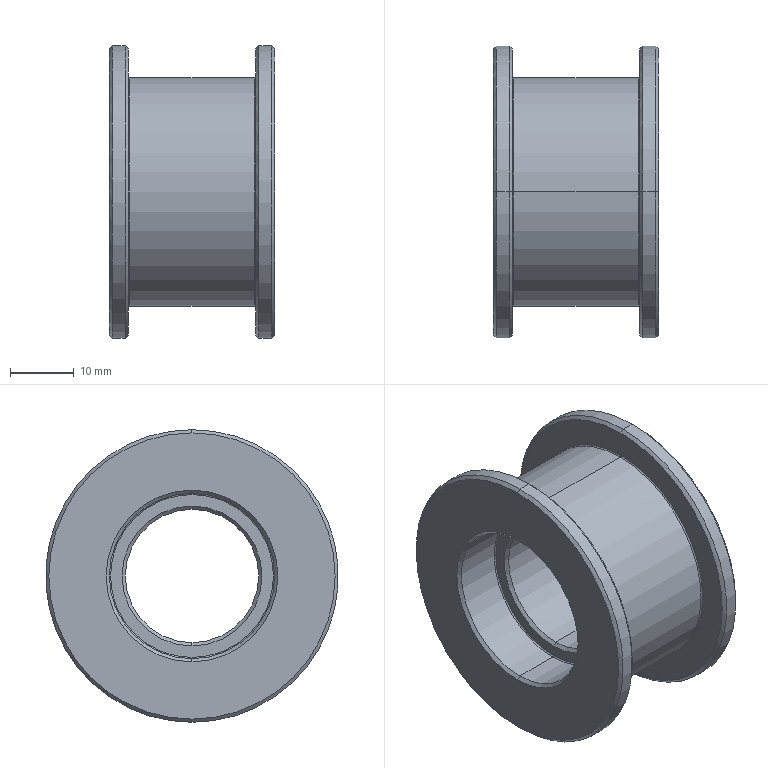Part | SolidWorks | features Chamfer 1, Fillet 1, Revolution 1 | 1 solid | 42 faces | box 26 x 46 x 46 mm | volume 18265 mm3 | cone 16 | cylinder 12 | torus 8 | plane 6 | commonest cylinder face diameters 26 x4 46 x4 21 x2 36 x2
STEP:
#1=CARTESIAN_POINT('',(-5.2,0.,13.));
#2=VERTEX_POINT('',#1);
#3=CARTESIAN_POINT('',(-5.2,0.,-13.));
#4=VERTEX_POINT('',#3);
#5=CARTESIAN_POINT('',(-5.2,0.,0.));
#6=DIRECTION('',(1.,0.,0.));
#7=DIRECTION('',(0.,0.,-1.));
#8=AXIS2_PLACEMENT_3D('',#5,#6,#7);
#9=CIRCLE('',#8,13.);
#10=EDGE_CURVE('',#2,#4,#9,.T.);
#11=ORIENTED_EDGE('',*,*,#10,.F.);
#12=CARTESIAN_POINT('',(-5.,0.,12.8));
#13=VERTEX_POINT('',#12);
#14=CARTESIAN_POINT('',(-5.2,0.,12.8));
#15=DIRECTION('',(0.,1.,0.));
#16=DIRECTION('',(0.,0.,1.));
#17=AXIS2_PLACEMENT_3D('',#14,#15,#16);
#18=CIRCLE('',#17,0.2);
#19=EDGE_CURVE('',#2,#13,#18,.T.);
#20=ORIENTED_EDGE('',*,*,#19,.T.);
#21=CARTESIAN_POINT('',(-5.,0.,-12.8));
#22=VERTEX_POINT('',#21);
#23=CARTESIAN_POINT('',(-5.,0.,0.));
#24=DIRECTION('',(-1.,0.,0.));
#25=DIRECTION('',(0.,0.,-1.));
#26=AXIS2_PLACEMENT_3D('',#23,#24,#25);
#27=CIRCLE('',#26,12.8);
#28=EDGE_CURVE('',#22,#13,#27,.T.);
#29=ORIENTED_EDGE('',*,*,#28,.F.);
#30=CARTESIAN_POINT('',(-5.2,0.,-12.8));
#31=DIRECTION('',(0.,-1.,0.));
#32=DIRECTION('',(0.,0.,-1.));
#33=AXIS2_PLACEMENT_3D('',#30,#31,#32);
#34=CIRCLE('',#33,0.2);
#35=EDGE_CURVE('',#4,#22,#34,.T.);
#36=ORIENTED_EDGE('',*,*,#35,.F.);
#37=EDGE_LOOP('',(#11,#20,#29,#36));
#38=FACE_OUTER_BOUND('',#37,.T.);
#39=CARTESIAN_POINT('',(-5.2,0.,0.));
#40=DIRECTION('',(1.,0.,0.));
#41=DIRECTION('',(0.,0.,-1.));
#42=AXIS2_PLACEMENT_3D('',#39,#40,#41);
#43=TOROIDAL_SURFACE('',#42,12.8,0.2);
#44=ADVANCED_FACE('',(#38),#43,.F.);
#45=CARTESIAN_POINT('',(10.,0.,18.2));
#46=VERTEX_POINT('',#45);
#47=CARTESIAN_POINT('',(10.,0.,-18.2));
#48=VERTEX_POINT('',#47);
#49=CARTESIAN_POINT('',(10.,0.,0.));
#50=DIRECTION('',(1.,0.,0.));
#51=DIRECTION('',(0.,0.,-1.));
#52=AXIS2_PLACEMENT_3D('',#49,#50,#51);
#53=CIRCLE('',#52,18.2);
#54=EDGE_CURVE('',#46,#48,#53,.T.);
#55=ORIENTED_EDGE('',*,*,#54,.F.);
#56=CARTESIAN_POINT('',(9.8,0.,18.));
#57=VERTEX_POINT('',#56);
#58=CARTESIAN_POINT('',(9.8,0.,18.2));
#59=DIRECTION('',(0.,1.,0.));
#60=DIRECTION('',(0.,0.,1.));
#61=AXIS2_PLACEMENT_3D('',#58,#59,#60);
#62=CIRCLE('',#61,0.2);
#63=EDGE_CURVE('',#46,#57,#62,.T.);
#64=ORIENTED_EDGE('',*,*,#63,.T.);
#65=CARTESIAN_POINT('',(9.8,0.,-18.));
#66=VERTEX_POINT('',#65);
#67=CARTESIAN_POINT('',(9.8,0.,0.));
#68=DIRECTION('',(-1.,0.,0.));
#69=DIRECTION('',(0.,0.,-1.));
#70=AXIS2_PLACEMENT_3D('',#67,#68,#69);
#71=CIRCLE('',#70,18.);
#72=EDGE_CURVE('',#66,#57,#71,.T.);
#73=ORIENTED_EDGE('',*,*,#72,.F.);
#74=CARTESIAN_POINT('',(9.8,0.,-18.2));
#75=DIRECTION('',(0.,-1.,0.));
#76=DIRECTION('',(0.,0.,-1.));
#77=AXIS2_PLACEMENT_3D('',#74,#75,#76);
#78=CIRCLE('',#77,0.2);
#79=EDGE_CURVE('',#48,#66,#78,.T.);
#80=ORIENTED_EDGE('',*,*,#79,.F.);
#81=EDGE_LOOP('',(#55,#64,#73,#80));
#82=FACE_OUTER_BOUND('',#81,.T.);
#83=CARTESIAN_POINT('',(9.8,0.,0.));
#84=DIRECTION('',(1.,0.,0.));
#85=DIRECTION('',(0.,0.,-1.));
#86=AXIS2_PLACEMENT_3D('',#83,#84,#85);
#87=TOROIDAL_SURFACE('',#86,18.2,0.2);
#88=ADVANCED_FACE('',(#82),#87,.F.);
#89=CARTESIAN_POINT('',(-10.,0.,-18.2));
#90=VERTEX_POINT('',#89);
#91=CARTESIAN_POINT('',(-10.,0.,18.2));
#92=VERTEX_POINT('',#91);
#93=CARTESIAN_POINT('',(-10.,0.,0.));
#94=DIRECTION('',(-1.,0.,0.));
#95=DIRECTION('',(0.,0.,1.));
#96=AXIS2_PLACEMENT_3D('',#93,#94,#95);
#97=CIRCLE('',#96,18.2);
#98=EDGE_CURVE('',#90,#92,#97,.T.);
#99=ORIENTED_EDGE('',*,*,#98,.F.);
#100=CARTESIAN_POINT('',(-9.8,0.,-18.));
#101=VERTEX_POINT('',#100);
#102=CARTESIAN_POINT('',(-9.8,0.,-18.2));
#103=DIRECTION('',(0.,1.,0.));
#104=DIRECTION('',(0.,0.,1.));
#105=AXIS2_PLACEMENT_3D('',#102,#103,#104);
#106=CIRCLE('',#105,0.2);
#107=EDGE_CURVE('',#90,#101,#106,.T.);
#108=ORIENTED_EDGE('',*,*,#107,.T.);
#109=CARTESIAN_POINT('',(-9.8,0.,18.));
#110=VERTEX_POINT('',#109);
#111=CARTESIAN_POINT('',(-9.8,0.,0.));
#112=DIRECTION('',(1.,0.,0.));
#113=DIRECTION('',(0.,0.,1.));
#114=AXIS2_PLACEMENT_3D('',#111,#112,#113);
#115=CIRCLE('',#114,18.);
#116=EDGE_CURVE('',#110,#101,#115,.T.);
#117=ORIENTED_EDGE('',*,*,#116,.F.);
#118=CARTESIAN_POINT('',(-9.8,0.,18.2));
#119=DIRECTION('',(0.,-1.,0.));
#120=DIRECTION('',(0.,0.,-1.));
#121=AXIS2_PLACEMENT_3D('',#118,#119,#120);
#122=CIRCLE('',#121,0.2);
#123=EDGE_CURVE('',#92,#110,#122,.T.);
#124=ORIENTED_EDGE('',*,*,#123,.F.);
#125=EDGE_LOOP('',(#99,#108,#117,#124));
#126=FACE_OUTER_BOUND('',#125,.T.);
#127=CARTESIAN_POINT('',(-9.8,0.,0.));
#128=DIRECTION('',(-1.,0.,0.));
#129=DIRECTION('',(0.,0.,1.));
#130=AXIS2_PLACEMENT_3D('',#127,#128,#129);
#131=TOROIDAL_SURFACE('',#130,18.2,0.2);
#132=ADVANCED_FACE('',(#126),#131,.F.);
#133=CARTESIAN_POINT('',(5.2,0.,-13.));
#134=VERTEX_POINT('',#133);
#135=CARTESIAN_POINT('',(5.2,0.,13.));
#136=VERTEX_POINT('',#135);
#137=CARTESIAN_POINT('',(5.2,0.,0.));
#138=DIRECTION('',(-1.,0.,0.));
#139=DIRECTION('',(0.,0.,1.));
#140=AXIS2_PLACEMENT_3D('',#137,#138,#139);
#141=CIRCLE('',#140,13.);
#142=EDGE_CURVE('',#134,#136,#141,.T.);
#143=ORIENTED_EDGE('',*,*,#142,.F.);
#144=CARTESIAN_POINT('',(5.,0.,-12.8));
#145=VERTEX_POINT('',#144);
#146=CARTESIAN_POINT('',(5.2,0.,-12.8));
#147=DIRECTION('',(0.,1.,0.));
#148=DIRECTION('',(0.,0.,1.));
#149=AXIS2_PLACEMENT_3D('',#146,#147,#148);
#150=CIRCLE('',#149,0.2);
#151=EDGE_CURVE('',#134,#145,#150,.T.);
#152=ORIENTED_EDGE('',*,*,#151,.T.);
#153=CARTESIAN_POINT('',(5.,0.,12.8));
#154=VERTEX_POINT('',#153);
#155=CARTESIAN_POINT('',(5.,0.,0.));
#156=DIRECTION('',(1.,0.,0.));
#157=DIRECTION('',(0.,0.,1.));
#158=AXIS2_PLACEMENT_3D('',#155,#156,#157);
#159=CIRCLE('',#158,12.8);
#160=EDGE_CURVE('',#154,#145,#159,.T.);
#161=ORIENTED_EDGE('',*,*,#160,.F.);
#162=CARTESIAN_POINT('',(5.2,0.,12.8));
#163=DIRECTION('',(0.,-1.,0.));
#164=DIRECTION('',(0.,0.,-1.));
#165=AXIS2_PLACEMENT_3D('',#162,#163,#164);
#166=CIRCLE('',#165,0.2);
#167=EDGE_CURVE('',#136,#154,#166,.T.);
#168=ORIENTED_EDGE('',*,*,#167,.F.);
#169=EDGE_LOOP('',(#143,#152,#161,#168));
#170=FACE_OUTER_BOUND('',#169,.T.);
#171=CARTESIAN_POINT('',(5.2,0.,0.));
#172=DIRECTION('',(-1.,0.,0.));
#173=DIRECTION('',(0.,0.,1.));
#174=AXIS2_PLACEMENT_3D('',#171,#172,#173);
#175=TOROIDAL_SURFACE('',#174,12.8,0.2);
#176=ADVANCED_FACE('',(#170),#175,.F.);
#177=CARTESIAN_POINT('',(-13.,0.,22.5));
#178=VERTEX_POINT('',#177);
#179=CARTESIAN_POINT('',(-13.,0.,-22.5));
#180=VERTEX_POINT('',#179);
#181=CARTESIAN_POINT('',(-13.,0.,0.));
#182=DIRECTION('',(-1.,0.,0.));
#183=DIRECTION('',(0.,0.,-1.));
#184=AXIS2_PLACEMENT_3D('',#181,#182,#183);
#185=CIRCLE('',#184,22.5);
#186=EDGE_CURVE('',#178,#180,#185,.T.);
#187=ORIENTED_EDGE('',*,*,#186,.F.);
#188=CARTESIAN_POINT('',(-12.5,0.,23.));
#189=VERTEX_POINT('',#188);
#190=CARTESIAN_POINT('',(-13.,0.,22.5));
#191=DIRECTION('',(0.7071,0.,0.7071));
#192=VECTOR('',#191,1000.);
#193=LINE('',#190,#192);
#194=EDGE_CURVE('',#178,#189,#193,.T.);
#195=ORIENTED_EDGE('',*,*,#194,.T.);
#196=CARTESIAN_POINT('',(-12.5,0.,-23.));
#197=VERTEX_POINT('',#196);
#198=CARTESIAN_POINT('',(-12.5,0.,0.));
#199=DIRECTION('',(1.,0.,0.));
#200=DIRECTION('',(0.,0.,-1.));
#201=AXIS2_PLACEMENT_3D('',#198,#199,#200);
#202=CIRCLE('',#201,23.);
#203=EDGE_CURVE('',#197,#189,#202,.T.);
#204=ORIENTED_EDGE('',*,*,#203,.F.);
#205=CARTESIAN_POINT('',(-13.,0.,-22.5));
#206=DIRECTION('',(0.7071,0.,-0.7071));
#207=VECTOR('',#206,1000.);
#208=LINE('',#205,#207);
#209=EDGE_CURVE('',#180,#197,#208,.T.);
#210=ORIENTED_EDGE('',*,*,#209,.F.);
#211=EDGE_LOOP('',(#187,#195,#204,#210));
#212=FACE_OUTER_BOUND('',#211,.T.);
#213=CARTESIAN_POINT('',(-13.,0.,0.));
#214=DIRECTION('',(1.,0.,0.));
#215=DIRECTION('',(0.,0.,-1.));
#216=AXIS2_PLACEMENT_3D('',#213,#214,#215);
#217=CONICAL_SURFACE('',#216,22.5,0.7854);
#218=ADVANCED_FACE('',(#212),#217,.T.);
#219=CARTESIAN_POINT('',(-12.5,0.,-13.));
#220=VERTEX_POINT('',#219);
#221=CARTESIAN_POINT('',(-12.5,0.,13.));
#222=VERTEX_POINT('',#221);
#223=CARTESIAN_POINT('',(-12.5,0.,0.));
#224=DIRECTION('',(-1.,0.,0.));
#225=DIRECTION('',(0.,0.,-1.));
#226=AXIS2_PLACEMENT_3D('',#223,#224,#225);
#227=CIRCLE('',#226,13.);
#228=EDGE_CURVE('',#220,#222,#227,.T.);
#229=ORIENTED_EDGE('',*,*,#228,.F.);
#230=CARTESIAN_POINT('',(-13.,0.,-13.5));
#231=VERTEX_POINT('',#230);
#232=CARTESIAN_POINT('',(-12.5,0.,-13.));
#233=DIRECTION('',(-0.7071,0.,-0.7071));
#234=VECTOR('',#233,1000.);
#235=LINE('',#232,#234);
#236=EDGE_CURVE('',#220,#231,#235,.T.);
#237=ORIENTED_EDGE('',*,*,#236,.T.);
#238=CARTESIAN_POINT('',(-13.,0.,13.5));
#239=VERTEX_POINT('',#238);
#240=CARTESIAN_POINT('',(-13.,0.,0.));
#241=DIRECTION('',(1.,0.,0.));
#242=DIRECTION('',(0.,0.,-1.));
#243=AXIS2_PLACEMENT_3D('',#240,#241,#242);
#244=CIRCLE('',#243,13.5);
#245=EDGE_CURVE('',#239,#231,#244,.T.);
#246=ORIENTED_EDGE('',*,*,#245,.F.);
#247=CARTESIAN_POINT('',(-12.5,0.,13.));
#248=DIRECTION('',(-0.7071,0.,0.7071));
#249=VECTOR('',#248,1000.);
#250=LINE('',#247,#249);
#251=EDGE_CURVE('',#222,#239,#250,.T.);
#252=ORIENTED_EDGE('',*,*,#251,.F.);
#253=EDGE_LOOP('',(#229,#237,#246,#252));
#254=FACE_OUTER_BOUND('',#253,.T.);
#255=CARTESIAN_POINT('',(-12.5,0.,0.));
#256=DIRECTION('',(-1.,0.,0.));
#257=DIRECTION('',(0.,0.,1.));
#258=AXIS2_PLACEMENT_3D('',#255,#256,#257);
#259=CONICAL_SURFACE('',#258,13.,0.7854);
#260=ADVANCED_FACE('',(#254),#259,.F.);
#261=CARTESIAN_POINT('',(-4.5,0.,-10.5));
#262=VERTEX_POINT('',#261);
#263=CARTESIAN_POINT('',(-4.5,0.,10.5));
#264=VERTEX_POINT('',#263);
#265=CARTESIAN_POINT('',(-4.5,0.,0.));
#266=DIRECTION('',(-1.,0.,0.));
#267=DIRECTION('',(0.,0.,-1.));
#268=AXIS2_PLACEMENT_3D('',#265,#266,#267);
#269=CIRCLE('',#268,10.5);
#270=EDGE_CURVE('',#262,#264,#269,.T.);
#271=ORIENTED_EDGE('',*,*,#270,.F.);
#272=CARTESIAN_POINT('',(-5.,0.,-11.));
#273=VERTEX_POINT('',#272);
#274=CARTESIAN_POINT('',(-4.5,0.,-10.5));
#275=DIRECTION('',(-0.7071,0.,-0.7071));
#276=VECTOR('',#275,1000.);
#277=LINE('',#274,#276);
#278=EDGE_CURVE('',#262,#273,#277,.T.);
#279=ORIENTED_EDGE('',*,*,#278,.T.);
#280=CARTESIAN_POINT('',(-5.,0.,11.));
#281=VERTEX_POINT('',#280);
#282=CARTESIAN_POINT('',(-5.,0.,0.));
#283=DIRECTION('',(1.,0.,0.));
#284=DIRECTION('',(0.,0.,-1.));
#285=AXIS2_PLACEMENT_3D('',#282,#283,#284);
#286=CIRCLE('',#285,11.);
#287=EDGE_CURVE('',#281,#273,#286,.T.);
#288=ORIENTED_EDGE('',*,*,#287,.F.);
#289=CARTESIAN_POINT('',(-4.5,0.,10.5));
#290=DIRECTION('',(-0.7071,0.,0.7071));
#291=VECTOR('',#290,1000.);
#292=LINE('',#289,#291);
#293=EDGE_CURVE('',#264,#281,#292,.T.);
#294=ORIENTED_EDGE('',*,*,#293,.F.);
#295=EDGE_LOOP('',(#271,#279,#288,#294));
#296=FACE_OUTER_BOUND('',#295,.T.);
#297=CARTESIAN_POINT('',(-4.5,0.,0.));
#298=DIRECTION('',(-1.,0.,0.));
#299=DIRECTION('',(0.,0.,1.));
#300=AXIS2_PLACEMENT_3D('',#297,#298,#299);
#301=CONICAL_SURFACE('',#300,10.5,0.7854);
#302=ADVANCED_FACE('',(#296),#301,.F.);
#303=CARTESIAN_POINT('',(-10.,0.,-22.5));
#304=VERTEX_POINT('',#303);
#305=CARTESIAN_POINT('',(-10.,0.,22.5));
#306=VERTEX_POINT('',#305);
#307=CARTESIAN_POINT('',(-10.,0.,0.));
#308=DIRECTION('',(1.,0.,0.));
#309=DIRECTION('',(0.,0.,1.));
#310=AXIS2_PLACEMENT_3D('',#307,#308,#309);
#311=CIRCLE('',#310,22.5);
#312=EDGE_CURVE('',#304,#306,#311,.T.);
#313=ORIENTED_EDGE('',*,*,#312,.F.);
#314=CARTESIAN_POINT('',(-10.5,0.,-23.));
#315=VERTEX_POINT('',#314);
#316=CARTESIAN_POINT('',(-10.5,0.,-23.));
#317=DIRECTION('',(-0.7071,0.,-0.7071));
#318=VECTOR('',#317,1000.);
#319=LINE('',#316,#318);
#320=EDGE_CURVE('',#304,#315,#319,.T.);
#321=ORIENTED_EDGE('',*,*,#320,.T.);
#322=CARTESIAN_POINT('',(-10.5,0.,23.));
#323=VERTEX_POINT('',#322);
#324=CARTESIAN_POINT('',(-10.5,0.,0.));
#325=DIRECTION('',(-1.,0.,0.));
#326=DIRECTION('',(0.,0.,1.));
#327=AXIS2_PLACEMENT_3D('',#324,#325,#326);
#328=CIRCLE('',#327,23.);
#329=EDGE_CURVE('',#323,#315,#328,.T.);
#330=ORIENTED_EDGE('',*,*,#329,.F.);
#331=CARTESIAN_POINT('',(-10.5,0.,23.));
#332=DIRECTION('',(-0.7071,0.,0.7071));
#333=VECTOR('',#332,1000.);
#334=LINE('',#331,#333);
#335=EDGE_CURVE('',#306,#323,#334,.T.);
#336=ORIENTED_EDGE('',*,*,#335,.F.);
#337=EDGE_LOOP('',(#313,#321,#330,#336));
#338=FACE_OUTER_BOUND('',#337,.T.);
#339=CARTESIAN_POINT('',(-10.5,0.,0.));
#340=DIRECTION('',(-1.,0.,0.));
#341=DIRECTION('',(0.,0.,1.));
#342=AXIS2_PLACEMENT_3D('',#339,#340,#341);
#343=CONICAL_SURFACE('',#342,23.,0.7854);
#344=ADVANCED_FACE('',(#338),#343,.T.);
#345=CARTESIAN_POINT('',(10.,0.,22.5));
#346=VERTEX_POINT('',#345);
#347=CARTESIAN_POINT('',(10.,0.,-22.5));
#348=VERTEX_POINT('',#347);
#349=CARTESIAN_POINT('',(10.,0.,0.));
#350=DIRECTION('',(-1.,0.,0.));
#351=DIRECTION('',(0.,0.,-1.));
#352=AXIS2_PLACEMENT_3D('',#349,#350,#351);
#353=CIRCLE('',#352,22.5);
#354=EDGE_CURVE('',#346,#348,#353,.T.);
#355=ORIENTED_EDGE('',*,*,#354,.F.);
#356=CARTESIAN_POINT('',(10.5,0.,23.));
#357=VERTEX_POINT('',#356);
#358=CARTESIAN_POINT('',(10.,0.,22.5));
#359=DIRECTION('',(0.7071,0.,0.7071));
#360=VECTOR('',#359,1000.);
#361=LINE('',#358,#360);
#362=EDGE_CURVE('',#346,#357,#361,.T.);
#363=ORIENTED_EDGE('',*,*,#362,.T.);
#364=CARTESIAN_POINT('',(10.5,0.,-23.));
#365=VERTEX_POINT('',#364);
#366=CARTESIAN_POINT('',(10.5,0.,0.));
#367=DIRECTION('',(1.,0.,0.));
#368=DIRECTION('',(0.,0.,-1.));
#369=AXIS2_PLACEMENT_3D('',#366,#367,#368);
#370=CIRCLE('',#369,23.);
#371=EDGE_CURVE('',#365,#357,#370,.T.);
#372=ORIENTED_EDGE('',*,*,#371,.F.);
#373=CARTESIAN_POINT('',(10.,0.,-22.5));
#374=DIRECTION('',(0.7071,0.,-0.7071));
#375=VECTOR('',#374,1000.);
#376=LINE('',#373,#375);
#377=EDGE_CURVE('',#348,#365,#376,.T.);
#378=ORIENTED_EDGE('',*,*,#377,.F.);
#379=EDGE_LOOP('',(#355,#363,#372,#378));
#380=FACE_OUTER_BOUND('',#379,.T.);
#381=CARTESIAN_POINT('',(10.,0.,0.));
#382=DIRECTION('',(1.,0.,0.));
#383=DIRECTION('',(0.,0.,-1.));
#384=AXIS2_PLACEMENT_3D('',#381,#382,#383);
#385=CONICAL_SURFACE('',#384,22.5,0.7854);
#386=ADVANCED_FACE('',(#380),#385,.T.);
#387=CARTESIAN_POINT('',(13.,0.,-22.5));
#388=VERTEX_POINT('',#387);
#389=CARTESIAN_POINT('',(13.,0.,22.5));
#390=VERTEX_POINT('',#389);
#391=CARTESIAN_POINT('',(13.,0.,0.));
#392=DIRECTION('',(1.,0.,0.));
#393=DIRECTION('',(0.,0.,1.));
#394=AXIS2_PLACEMENT_3D('',#391,#392,#393);
#395=CIRCLE('',#394,22.5);
#396=EDGE_CURVE('',#388,#390,#395,.T.);
#397=ORIENTED_EDGE('',*,*,#396,.F.);
#398=CARTESIAN_POINT('',(12.5,0.,-23.));
#399=VERTEX_POINT('',#398);
#400=CARTESIAN_POINT('',(12.5,0.,-23.));
#401=DIRECTION('',(-0.7071,0.,-0.7071));
#402=VECTOR('',#401,1000.);
#403=LINE('',#400,#402);
#404=EDGE_CURVE('',#388,#399,#403,.T.);
#405=ORIENTED_EDGE('',*,*,#404,.T.);
#406=CARTESIAN_POINT('',(12.5,0.,23.));
#407=VERTEX_POINT('',#406);
#408=CARTESIAN_POINT('',(12.5,0.,0.));
#409=DIRECTION('',(-1.,0.,0.));
#410=DIRECTION('',(0.,0.,1.));
#411=AXIS2_PLACEMENT_3D('',#408,#409,#410);
#412=CIRCLE('',#411,23.);
#413=EDGE_CURVE('',#407,#399,#412,.T.);
#414=ORIENTED_EDGE('',*,*,#413,.F.);
#415=CARTESIAN_POINT('',(12.5,0.,23.));
#416=DIRECTION('',(-0.7071,0.,0.7071));
#417=VECTOR('',#416,1000.);
#418=LINE('',#415,#417);
#419=EDGE_CURVE('',#390,#407,#418,.T.);
#420=ORIENTED_EDGE('',*,*,#419,.F.);
#421=EDGE_LOOP('',(#397,#405,#414,#420));
#422=FACE_OUTER_BOUND('',#421,.T.);
#423=CARTESIAN_POINT('',(12.5,0.,0.));
#424=DIRECTION('',(-1.,0.,0.));
#425=DIRECTION('',(0.,0.,1.));
#426=AXIS2_PLACEMENT_3D('',#423,#424,#425);
#427=CONICAL_SURFACE('',#426,23.,0.7854);
#428=ADVANCED_FACE('',(#422),#427,.T.);
#429=CARTESIAN_POINT('',(12.5,0.,13.));
#430=VERTEX_POINT('',#429);
#431=CARTESIAN_POINT('',(12.5,0.,-13.));
#432=VERTEX_POINT('',#431);
#433=CARTESIAN_POINT('',(12.5,0.,0.));
#434=DIRECTION('',(1.,0.,0.));
#435=DIRECTION('',(0.,0.,1.));
#436=AXIS2_PLACEMENT_3D('',#433,#434,#435);
#437=CIRCLE('',#436,13.);
#438=EDGE_CURVE('',#430,#432,#437,.T.);
#439=ORIENTED_EDGE('',*,*,#438,.F.);
#440=CARTESIAN_POINT('',(13.,0.,13.5));
#441=VERTEX_POINT('',#440);
#442=CARTESIAN_POINT('',(13.,0.,13.5));
#443=DIRECTION('',(0.7071,0.,0.7071));
#444=VECTOR('',#443,1000.);
#445=LINE('',#442,#444);
#446=EDGE_CURVE('',#430,#441,#445,.T.);
#447=ORIENTED_EDGE('',*,*,#446,.T.);
#448=CARTESIAN_POINT('',(13.,0.,-13.5));
#449=VERTEX_POINT('',#448);
#450=CARTESIAN_POINT('',(13.,0.,0.));
#451=DIRECTION('',(-1.,0.,0.));
#452=DIRECTION('',(0.,0.,1.));
#453=AXIS2_PLACEMENT_3D('',#450,#451,#452);
#454=CIRCLE('',#453,13.5);
#455=EDGE_CURVE('',#449,#441,#454,.T.);
#456=ORIENTED_EDGE('',*,*,#455,.F.);
#457=CARTESIAN_POINT('',(13.,0.,-13.5));
#458=DIRECTION('',(0.7071,0.,-0.7071));
#459=VECTOR('',#458,1000.);
#460=LINE('',#457,#459);
#461=EDGE_CURVE('',#432,#449,#460,.T.);
#462=ORIENTED_EDGE('',*,*,#461,.F.);
#463=EDGE_LOOP('',(#439,#447,#456,#462));
#464=FACE_OUTER_BOUND('',#463,.T.);
#465=CARTESIAN_POINT('',(13.,0.,0.));
#466=DIRECTION('',(1.,0.,0.));
#467=DIRECTION('',(0.,0.,-1.));
#468=AXIS2_PLACEMENT_3D('',#465,#466,#467);
#469=CONICAL_SURFACE('',#468,13.5,0.7854);
#470=ADVANCED_FACE('',(#464),#469,.F.);
#471=CARTESIAN_POINT('',(4.5,0.,10.5));
#472=VERTEX_POINT('',#471);
#473=CARTESIAN_POINT('',(4.5,0.,-10.5));
#474=VERTEX_POINT('',#473);
#475=CARTESIAN_POINT('',(4.5,0.,0.));
#476=DIRECTION('',(1.,0.,0.));
#477=DIRECTION('',(0.,0.,1.));
#478=AXIS2_PLACEMENT_3D('',#475,#476,#477);
#479=CIRCLE('',#478,10.5);
#480=EDGE_CURVE('',#472,#474,#479,.T.);
#481=ORIENTED_EDGE('',*,*,#480,.F.);
#482=CARTESIAN_POINT('',(5.,0.,11.));
#483=VERTEX_POINT('',#482);
#484=CARTESIAN_POINT('',(5.,0.,11.));
#485=DIRECTION('',(0.7071,0.,0.7071));
#486=VECTOR('',#485,1000.);
#487=LINE('',#484,#486);
#488=EDGE_CURVE('',#472,#483,#487,.T.);
#489=ORIENTED_EDGE('',*,*,#488,.T.);
#490=CARTESIAN_POINT('',(5.,0.,-11.));
#491=VERTEX_POINT('',#490);
#492=CARTESIAN_POINT('',(5.,0.,0.));
#493=DIRECTION('',(-1.,0.,0.));
#494=DIRECTION('',(0.,0.,1.));
#495=AXIS2_PLACEMENT_3D('',#492,#493,#494);
#496=CIRCLE('',#495,11.);
#497=EDGE_CURVE('',#491,#483,#496,.T.);
#498=ORIENTED_EDGE('',*,*,#497,.F.);
#499=CARTESIAN_POINT('',(5.,0.,-11.));
#500=DIRECTION('',(0.7071,0.,-0.7071));
#501=VECTOR('',#500,1000.);
#502=LINE('',#499,#501);
#503=EDGE_CURVE('',#474,#491,#502,.T.);
#504=ORIENTED_EDGE('',*,*,#503,.F.);
#505=EDGE_LOOP('',(#481,#489,#498,#504));
#506=FACE_OUTER_BOUND('',#505,.T.);
#507=CARTESIAN_POINT('',(5.,0.,0.));
#508=DIRECTION('',(1.,0.,0.));
#509=DIRECTION('',(0.,0.,-1.));
#510=AXIS2_PLACEMENT_3D('',#507,#508,#509);
#511=CONICAL_SURFACE('',#510,11.,0.7854);
#512=ADVANCED_FACE('',(#506),#511,.F.);
#513=ORIENTED_EDGE('',*,*,#480,.T.);
#514=CARTESIAN_POINT('',(0.,0.,-10.5));
#515=DIRECTION('',(-1.,0.,0.));
#516=VECTOR('',#515,1000.);
#517=LINE('',#514,#516);
#518=EDGE_CURVE('',#474,#262,#517,.T.);
#519=ORIENTED_EDGE('',*,*,#518,.T.);
#520=ORIENTED_EDGE('',*,*,#270,.T.);
#521=CARTESIAN_POINT('',(0.,0.,10.5));
#522=DIRECTION('',(-1.,0.,0.));
#523=VECTOR('',#522,1000.);
#524=LINE('',#521,#523);
#525=EDGE_CURVE('',#472,#264,#524,.T.);
#526=ORIENTED_EDGE('',*,*,#525,.F.);
#527=EDGE_LOOP('',(#513,#519,#520,#526));
#528=FACE_OUTER_BOUND('',#527,.T.);
#529=CARTESIAN_POINT('',(0.,0.,0.));
#530=DIRECTION('',(-1.,0.,0.));
#531=DIRECTION('',(0.,0.,1.));
#532=AXIS2_PLACEMENT_3D('',#529,#530,#531);
#533=CYLINDRICAL_SURFACE('',#532,10.5);
#534=ADVANCED_FACE('',(#528),#533,.F.);
#535=ORIENTED_EDGE('',*,*,#438,.T.);
#536=CARTESIAN_POINT('',(0.,0.,-13.));
#537=DIRECTION('',(-1.,0.,0.));
#538=VECTOR('',#537,1000.);
#539=LINE('',#536,#538);
#540=EDGE_CURVE('',#432,#134,#539,.T.);
#541=ORIENTED_EDGE('',*,*,#540,.T.);
#542=ORIENTED_EDGE('',*,*,#142,.T.);
#543=CARTESIAN_POINT('',(0.,0.,13.));
#544=DIRECTION('',(-1.,0.,0.));
#545=VECTOR('',#544,1000.);
#546=LINE('',#543,#545);
#547=EDGE_CURVE('',#430,#136,#546,.T.);
#548=ORIENTED_EDGE('',*,*,#547,.F.);
#549=EDGE_LOOP('',(#535,#541,#542,#548));
#550=FACE_OUTER_BOUND('',#549,.T.);
#551=CARTESIAN_POINT('',(0.,0.,0.));
#552=DIRECTION('',(-1.,0.,0.));
#553=DIRECTION('',(0.,0.,1.));
#554=AXIS2_PLACEMENT_3D('',#551,#552,#553);
#555=CYLINDRICAL_SURFACE('',#554,13.);
#556=ADVANCED_FACE('',(#550),#555,.F.);
#557=ORIENTED_EDGE('',*,*,#413,.T.);
#558=CARTESIAN_POINT('',(0.,0.,-23.));
#559=DIRECTION('',(-1.,0.,0.));
#560=VECTOR('',#559,1000.);
#561=LINE('',#558,#560);
#562=EDGE_CURVE('',#399,#365,#561,.T.);
#563=ORIENTED_EDGE('',*,*,#562,.T.);
#564=ORIENTED_EDGE('',*,*,#371,.T.);
#565=CARTESIAN_POINT('',(0.,0.,23.));
#566=DIRECTION('',(-1.,0.,0.));
#567=VECTOR('',#566,1000.);
#568=LINE('',#565,#567);
#569=EDGE_CURVE('',#407,#357,#568,.T.);
#570=ORIENTED_EDGE('',*,*,#569,.F.);
#571=EDGE_LOOP('',(#557,#563,#564,#570));
#572=FACE_OUTER_BOUND('',#571,.T.);
#573=CARTESIAN_POINT('',(0.,0.,0.));
#574=DIRECTION('',(-1.,0.,0.));
#575=DIRECTION('',(0.,0.,1.));
#576=AXIS2_PLACEMENT_3D('',#573,#574,#575);
#577=CYLINDRICAL_SURFACE('',#576,23.);
#578=ADVANCED_FACE('',(#572),#577,.T.);
#579=CARTESIAN_POINT('',(9.8,0.,0.));
#580=DIRECTION('',(-1.,0.,0.));
#581=DIRECTION('',(0.,0.,-1.));
#582=AXIS2_PLACEMENT_3D('',#579,#580,#581);
#583=CIRCLE('',#582,18.);
#584=EDGE_CURVE('',#57,#66,#583,.T.);
#585=ORIENTED_EDGE('',*,*,#584,.T.);
#586=CARTESIAN_POINT('',(0.,0.,-18.));
#587=DIRECTION('',(-1.,0.,0.));
#588=VECTOR('',#587,1000.);
#589=LINE('',#586,#588);
#590=EDGE_CURVE('',#66,#101,#589,.T.);
#591=ORIENTED_EDGE('',*,*,#590,.T.);
#592=CARTESIAN_POINT('',(-9.8,0.,0.));
#593=DIRECTION('',(1.,0.,0.));
#594=DIRECTION('',(0.,0.,1.));
#595=AXIS2_PLACEMENT_3D('',#592,#593,#594);
#596=CIRCLE('',#595,18.);
#597=EDGE_CURVE('',#101,#110,#596,.T.);
#598=ORIENTED_EDGE('',*,*,#597,.T.);
#599=CARTESIAN_POINT('',(0.,0.,18.));
#600=DIRECTION('',(-1.,0.,0.));
#601=VECTOR('',#600,1000.);
#602=LINE('',#599,#601);
#603=EDGE_CURVE('',#57,#110,#602,.T.);
#604=ORIENTED_EDGE('',*,*,#603,.F.);
#605=EDGE_LOOP('',(#585,#591,#598,#604));
#606=FACE_OUTER_BOUND('',#605,.T.);
#607=CARTESIAN_POINT('',(0.,0.,0.));
#608=DIRECTION('',(-1.,0.,0.));
#609=DIRECTION('',(0.,0.,1.));
#610=AXIS2_PLACEMENT_3D('',#607,#608,#609);
#611=CYLINDRICAL_SURFACE('',#610,18.);
#612=ADVANCED_FACE('',(#606),#611,.T.);
#613=ORIENTED_EDGE('',*,*,#329,.T.);
#614=CARTESIAN_POINT('',(0.,0.,-23.));
#615=DIRECTION('',(-1.,0.,0.));
#616=VECTOR('',#615,1000.);
#617=LINE('',#614,#616);
#618=EDGE_CURVE('',#315,#197,#617,.T.);
#619=ORIENTED_EDGE('',*,*,#618,.T.);
#620=ORIENTED_EDGE('',*,*,#203,.T.);
#621=CARTESIAN_POINT('',(0.,0.,23.));
#622=DIRECTION('',(-1.,0.,0.));
#623=VECTOR('',#622,1000.);
#624=LINE('',#621,#623);
#625=EDGE_CURVE('',#323,#189,#624,.T.);
#626=ORIENTED_EDGE('',*,*,#625,.F.);
#627=EDGE_LOOP('',(#613,#619,#620,#626));
#628=FACE_OUTER_BOUND('',#627,.T.);
#629=CARTESIAN_POINT('',(0.,0.,0.));
#630=DIRECTION('',(-1.,0.,0.));
#631=DIRECTION('',(0.,0.,1.));
#632=AXIS2_PLACEMENT_3D('',#629,#630,#631);
#633=CYLINDRICAL_SURFACE('',#632,23.);
#634=ADVANCED_FACE('',(#628),#633,.T.);
#635=ORIENTED_EDGE('',*,*,#10,.T.);
#636=CARTESIAN_POINT('',(0.,0.,-13.));
#637=DIRECTION('',(-1.,0.,0.));
#638=VECTOR('',#637,1000.);
#639=LINE('',#636,#638);
#640=EDGE_CURVE('',#4,#220,#639,.T.);
#641=ORIENTED_EDGE('',*,*,#640,.T.);
#642=ORIENTED_EDGE('',*,*,#228,.T.);
#643=CARTESIAN_POINT('',(0.,0.,13.));
#644=DIRECTION('',(-1.,0.,0.));
#645=VECTOR('',#644,1000.);
#646=LINE('',#643,#645);
#647=EDGE_CURVE('',#2,#222,#646,.T.);
#648=ORIENTED_EDGE('',*,*,#647,.F.);
#649=EDGE_LOOP('',(#635,#641,#642,#648));
#650=FACE_OUTER_BOUND('',#649,.T.);
#651=CARTESIAN_POINT('',(0.,0.,0.));
#652=DIRECTION('',(-1.,0.,0.));
#653=DIRECTION('',(0.,0.,1.));
#654=AXIS2_PLACEMENT_3D('',#651,#652,#653);
#655=CYLINDRICAL_SURFACE('',#654,13.);
#656=ADVANCED_FACE('',(#650),#655,.F.);
#657=ORIENTED_EDGE('',*,*,#640,.F.);
#658=CARTESIAN_POINT('',(-5.2,0.,0.));
#659=DIRECTION('',(1.,0.,0.));
#660=DIRECTION('',(0.,0.,-1.));
#661=AXIS2_PLACEMENT_3D('',#658,#659,#660);
#662=CIRCLE('',#661,13.);
#663=EDGE_CURVE('',#4,#2,#662,.T.);
#664=ORIENTED_EDGE('',*,*,#663,.T.);
#665=ORIENTED_EDGE('',*,*,#647,.T.);
#666=CARTESIAN_POINT('',(-12.5,0.,0.));
#667=DIRECTION('',(-1.,0.,0.));
#668=DIRECTION('',(0.,0.,-1.));
#669=AXIS2_PLACEMENT_3D('',#666,#667,#668);
#670=CIRCLE('',#669,13.);
#671=EDGE_CURVE('',#222,#220,#670,.T.);
#672=ORIENTED_EDGE('',*,*,#671,.T.);
#673=EDGE_LOOP('',(#657,#664,#665,#672));
#674=FACE_OUTER_BOUND('',#673,.T.);
#675=CARTESIAN_POINT('',(0.,0.,0.));
#676=DIRECTION('',(-1.,0.,0.));
#677=DIRECTION('',(0.,0.,1.));
#678=AXIS2_PLACEMENT_3D('',#675,#676,#677);
#679=CYLINDRICAL_SURFACE('',#678,13.);
#680=ADVANCED_FACE('',(#674),#679,.F.);
#681=ORIENTED_EDGE('',*,*,#245,.T.);
#682=CARTESIAN_POINT('',(-13.,0.,0.));
#683=DIRECTION('',(1.,0.,0.));
#684=DIRECTION('',(0.,0.,-1.));
#685=AXIS2_PLACEMENT_3D('',#682,#683,#684);
#686=CIRCLE('',#685,13.5);
#687=EDGE_CURVE('',#231,#239,#686,.T.);
#688=ORIENTED_EDGE('',*,*,#687,.T.);
#689=EDGE_LOOP('',(#681,#688));
#690=FACE_BOUND('',#689,.T.);
#691=CARTESIAN_POINT('',(-13.,0.,0.));
#692=DIRECTION('',(-1.,0.,0.));
#693=DIRECTION('',(0.,0.,-1.));
#694=AXIS2_PLACEMENT_3D('',#691,#692,#693);
#695=CIRCLE('',#694,22.5);
#696=EDGE_CURVE('',#180,#178,#695,.T.);
#697=ORIENTED_EDGE('',*,*,#696,.T.);
#698=ORIENTED_EDGE('',*,*,#186,.T.);
#699=EDGE_LOOP('',(#697,#698));
#700=FACE_OUTER_BOUND('',#699,.T.);
#701=CARTESIAN_POINT('',(-13.,13.,0.));
#702=DIRECTION('',(1.,0.,0.));
#703=DIRECTION('',(0.,0.,-1.));
#704=AXIS2_PLACEMENT_3D('',#701,#702,#703);
#705=PLANE('',#704);
#706=ADVANCED_FACE('',(#690,#700),#705,.F.);
#707=ORIENTED_EDGE('',*,*,#618,.F.);
#708=CARTESIAN_POINT('',(-10.5,0.,0.));
#709=DIRECTION('',(-1.,0.,0.));
#710=DIRECTION('',(0.,0.,1.));
#711=AXIS2_PLACEMENT_3D('',#708,#709,#710);
#712=CIRCLE('',#711,23.);
#713=EDGE_CURVE('',#315,#323,#712,.T.);
#714=ORIENTED_EDGE('',*,*,#713,.T.);
#715=ORIENTED_EDGE('',*,*,#625,.T.);
#716=CARTESIAN_POINT('',(-12.5,0.,0.));
#717=DIRECTION('',(1.,0.,0.));
#718=DIRECTION('',(0.,0.,-1.));
#719=AXIS2_PLACEMENT_3D('',#716,#717,#718);
#720=CIRCLE('',#719,23.);
#721=EDGE_CURVE('',#189,#197,#720,.T.);
#722=ORIENTED_EDGE('',*,*,#721,.T.);
#723=EDGE_LOOP('',(#707,#714,#715,#722));
#724=FACE_OUTER_BOUND('',#723,.T.);
#725=CARTESIAN_POINT('',(0.,0.,0.));
#726=DIRECTION('',(-1.,0.,0.));
#727=DIRECTION('',(0.,0.,1.));
#728=AXIS2_PLACEMENT_3D('',#725,#726,#727);
#729=CYLINDRICAL_SURFACE('',#728,23.);
#730=ADVANCED_FACE('',(#724),#729,.T.);
#731=CARTESIAN_POINT('',(-10.,0.,0.));
#732=DIRECTION('',(-1.,0.,0.));
#733=DIRECTION('',(0.,0.,1.));
#734=AXIS2_PLACEMENT_3D('',#731,#732,#733);
#735=CIRCLE('',#734,18.2);
#736=EDGE_CURVE('',#92,#90,#735,.T.);
#737=ORIENTED_EDGE('',*,*,#736,.T.);
#738=ORIENTED_EDGE('',*,*,#98,.T.);
#739=EDGE_LOOP('',(#737,#738));
#740=FACE_BOUND('',#739,.T.);
#741=CARTESIAN_POINT('',(-10.,0.,0.));
#742=DIRECTION('',(1.,0.,0.));
#743=DIRECTION('',(0.,0.,1.));
#744=AXIS2_PLACEMENT_3D('',#741,#742,#743);
#745=CIRCLE('',#744,22.5);
#746=EDGE_CURVE('',#306,#304,#745,.T.);
#747=ORIENTED_EDGE('',*,*,#746,.T.);
#748=ORIENTED_EDGE('',*,*,#312,.T.);
#749=EDGE_LOOP('',(#747,#748));
#750=FACE_OUTER_BOUND('',#749,.T.);
#751=CARTESIAN_POINT('',(-10.,23.,0.));
#752=DIRECTION('',(-1.,0.,0.));
#753=DIRECTION('',(0.,0.,1.));
#754=AXIS2_PLACEMENT_3D('',#751,#752,#753);
#755=PLANE('',#754);
#756=ADVANCED_FACE('',(#740,#750),#755,.F.);
#757=ORIENTED_EDGE('',*,*,#590,.F.);
#758=ORIENTED_EDGE('',*,*,#72,.T.);
#759=ORIENTED_EDGE('',*,*,#603,.T.);
#760=ORIENTED_EDGE('',*,*,#116,.T.);
#761=EDGE_LOOP('',(#757,#758,#759,#760));
#762=FACE_OUTER_BOUND('',#761,.T.);
#763=CARTESIAN_POINT('',(0.,0.,0.));
#764=DIRECTION('',(-1.,0.,0.));
#765=DIRECTION('',(0.,0.,1.));
#766=AXIS2_PLACEMENT_3D('',#763,#764,#765);
#767=CYLINDRICAL_SURFACE('',#766,18.);
#768=ADVANCED_FACE('',(#762),#767,.T.);
#769=CARTESIAN_POINT('',(10.,0.,0.));
#770=DIRECTION('',(1.,0.,0.));
#771=DIRECTION('',(0.,0.,-1.));
#772=AXIS2_PLACEMENT_3D('',#769,#770,#771);
#773=CIRCLE('',#772,18.2);
#774=EDGE_CURVE('',#48,#46,#773,.T.);
#775=ORIENTED_EDGE('',*,*,#774,.T.);
#776=ORIENTED_EDGE('',*,*,#54,.T.);
#777=EDGE_LOOP('',(#775,#776));
#778=FACE_BOUND('',#777,.T.);
#779=CARTESIAN_POINT('',(10.,0.,0.));
#780=DIRECTION('',(-1.,0.,0.));
#781=DIRECTION('',(0.,0.,-1.));
#782=AXIS2_PLACEMENT_3D('',#779,#780,#781);
#783=CIRCLE('',#782,22.5);
#784=EDGE_CURVE('',#348,#346,#783,.T.);
#785=ORIENTED_EDGE('',*,*,#784,.T.);
#786=ORIENTED_EDGE('',*,*,#354,.T.);
#787=EDGE_LOOP('',(#785,#786));
#788=FACE_OUTER_BOUND('',#787,.T.);
#789=CARTESIAN_POINT('',(10.,23.,0.));
#790=DIRECTION('',(1.,0.,0.));
#791=DIRECTION('',(0.,0.,-1.));
#792=AXIS2_PLACEMENT_3D('',#789,#790,#791);
#793=PLANE('',#792);
#794=ADVANCED_FACE('',(#778,#788),#793,.F.);
#795=ORIENTED_EDGE('',*,*,#562,.F.);
#796=CARTESIAN_POINT('',(12.5,0.,0.));
#797=DIRECTION('',(-1.,0.,0.));
#798=DIRECTION('',(0.,0.,1.));
#799=AXIS2_PLACEMENT_3D('',#796,#797,#798);
#800=CIRCLE('',#799,23.);
#801=EDGE_CURVE('',#399,#407,#800,.T.);
#802=ORIENTED_EDGE('',*,*,#801,.T.);
#803=ORIENTED_EDGE('',*,*,#569,.T.);
#804=CARTESIAN_POINT('',(10.5,0.,0.));
#805=DIRECTION('',(1.,0.,0.));
#806=DIRECTION('',(0.,0.,-1.));
#807=AXIS2_PLACEMENT_3D('',#804,#805,#806);
#808=CIRCLE('',#807,23.);
#809=EDGE_CURVE('',#357,#365,#808,.T.);
#810=ORIENTED_EDGE('',*,*,#809,.T.);
#811=EDGE_LOOP('',(#795,#802,#803,#810));
#812=FACE_OUTER_BOUND('',#811,.T.);
#813=CARTESIAN_POINT('',(0.,0.,0.));
#814=DIRECTION('',(-1.,0.,0.));
#815=DIRECTION('',(0.,0.,1.));
#816=AXIS2_PLACEMENT_3D('',#813,#814,#815);
#817=CYLINDRICAL_SURFACE('',#816,23.);
#818=ADVANCED_FACE('',(#812),#817,.T.);
#819=ORIENTED_EDGE('',*,*,#455,.T.);
#820=CARTESIAN_POINT('',(13.,0.,0.));
#821=DIRECTION('',(-1.,0.,0.));
#822=DIRECTION('',(0.,0.,1.));
#823=AXIS2_PLACEMENT_3D('',#820,#821,#822);
#824=CIRCLE('',#823,13.5);
#825=EDGE_CURVE('',#441,#449,#824,.T.);
#826=ORIENTED_EDGE('',*,*,#825,.T.);
#827=EDGE_LOOP('',(#819,#826));
#828=FACE_BOUND('',#827,.T.);
#829=CARTESIAN_POINT('',(13.,0.,0.));
#830=DIRECTION('',(1.,0.,0.));
#831=DIRECTION('',(0.,0.,1.));
#832=AXIS2_PLACEMENT_3D('',#829,#830,#831);
#833=CIRCLE('',#832,22.5);
#834=EDGE_CURVE('',#390,#388,#833,.T.);
#835=ORIENTED_EDGE('',*,*,#834,.T.);
#836=ORIENTED_EDGE('',*,*,#396,.T.);
#837=EDGE_LOOP('',(#835,#836));
#838=FACE_OUTER_BOUND('',#837,.T.);
#839=CARTESIAN_POINT('',(13.,13.,0.));
#840=DIRECTION('',(-1.,0.,0.));
#841=DIRECTION('',(0.,0.,1.));
#842=AXIS2_PLACEMENT_3D('',#839,#840,#841);
#843=PLANE('',#842);
#844=ADVANCED_FACE('',(#828,#838),#843,.F.);
#845=ORIENTED_EDGE('',*,*,#540,.F.);
#846=CARTESIAN_POINT('',(12.5,0.,0.));
#847=DIRECTION('',(1.,0.,0.));
#848=DIRECTION('',(0.,0.,1.));
#849=AXIS2_PLACEMENT_3D('',#846,#847,#848);
#850=CIRCLE('',#849,13.);
#851=EDGE_CURVE('',#432,#430,#850,.T.);
#852=ORIENTED_EDGE('',*,*,#851,.T.);
#853=ORIENTED_EDGE('',*,*,#547,.T.);
#854=CARTESIAN_POINT('',(5.2,0.,0.));
#855=DIRECTION('',(-1.,0.,0.));
#856=DIRECTION('',(0.,0.,1.));
#857=AXIS2_PLACEMENT_3D('',#854,#855,#856);
#858=CIRCLE('',#857,13.);
#859=EDGE_CURVE('',#136,#134,#858,.T.);
#860=ORIENTED_EDGE('',*,*,#859,.T.);
#861=EDGE_LOOP('',(#845,#852,#853,#860));
#862=FACE_OUTER_BOUND('',#861,.T.);
#863=CARTESIAN_POINT('',(0.,0.,0.));
#864=DIRECTION('',(-1.,0.,0.));
#865=DIRECTION('',(0.,0.,1.));
#866=AXIS2_PLACEMENT_3D('',#863,#864,#865);
#867=CYLINDRICAL_SURFACE('',#866,13.);
#868=ADVANCED_FACE('',(#862),#867,.F.);
#869=ORIENTED_EDGE('',*,*,#160,.T.);
#870=CARTESIAN_POINT('',(5.,0.,0.));
#871=DIRECTION('',(1.,0.,0.));
#872=DIRECTION('',(0.,0.,1.));
#873=AXIS2_PLACEMENT_3D('',#870,#871,#872);
#874=CIRCLE('',#873,12.8);
#875=EDGE_CURVE('',#145,#154,#874,.T.);
#876=ORIENTED_EDGE('',*,*,#875,.T.);
#877=EDGE_LOOP('',(#869,#876));
#878=FACE_OUTER_BOUND('',#877,.T.);
#879=ORIENTED_EDGE('',*,*,#497,.T.);
#880=CARTESIAN_POINT('',(5.,0.,0.));
#881=DIRECTION('',(-1.,0.,0.));
#882=DIRECTION('',(0.,0.,1.));
#883=AXIS2_PLACEMENT_3D('',#880,#881,#882);
#884=CIRCLE('',#883,11.);
#885=EDGE_CURVE('',#483,#491,#884,.T.);
#886=ORIENTED_EDGE('',*,*,#885,.T.);
#887=EDGE_LOOP('',(#879,#886));
#888=FACE_BOUND('',#887,.T.);
#889=CARTESIAN_POINT('',(5.,13.,0.));
#890=DIRECTION('',(-1.,0.,0.));
#891=DIRECTION('',(0.,0.,1.));
#892=AXIS2_PLACEMENT_3D('',#889,#890,#891);
#893=PLANE('',#892);
#894=ADVANCED_FACE('',(#878,#888),#893,.F.);
#895=ORIENTED_EDGE('',*,*,#518,.F.);
#896=CARTESIAN_POINT('',(4.5,0.,0.));
#897=DIRECTION('',(1.,0.,0.));
#898=DIRECTION('',(0.,0.,1.));
#899=AXIS2_PLACEMENT_3D('',#896,#897,#898);
#900=CIRCLE('',#899,10.5);
#901=EDGE_CURVE('',#474,#472,#900,.T.);
#902=ORIENTED_EDGE('',*,*,#901,.T.);
#903=ORIENTED_EDGE('',*,*,#525,.T.);
#904=CARTESIAN_POINT('',(-4.5,0.,0.));
#905=DIRECTION('',(-1.,0.,0.));
#906=DIRECTION('',(0.,0.,-1.));
#907=AXIS2_PLACEMENT_3D('',#904,#905,#906);
#908=CIRCLE('',#907,10.5);
#909=EDGE_CURVE('',#264,#262,#908,.T.);
#910=ORIENTED_EDGE('',*,*,#909,.T.);
#911=EDGE_LOOP('',(#895,#902,#903,#910));
#912=FACE_OUTER_BOUND('',#911,.T.);
#913=CARTESIAN_POINT('',(0.,0.,0.));
#914=DIRECTION('',(-1.,0.,0.));
#915=DIRECTION('',(0.,0.,1.));
#916=AXIS2_PLACEMENT_3D('',#913,#914,#915);
#917=CYLINDRICAL_SURFACE('',#916,10.5);
#918=ADVANCED_FACE('',(#912),#917,.F.);
#919=ORIENTED_EDGE('',*,*,#28,.T.);
#920=CARTESIAN_POINT('',(-5.,0.,0.));
#921=DIRECTION('',(-1.,0.,0.));
#922=DIRECTION('',(0.,0.,-1.));
#923=AXIS2_PLACEMENT_3D('',#920,#921,#922);
#924=CIRCLE('',#923,12.8);
#925=EDGE_CURVE('',#13,#22,#924,.T.);
#926=ORIENTED_EDGE('',*,*,#925,.T.);
#927=EDGE_LOOP('',(#919,#926));
#928=FACE_OUTER_BOUND('',#927,.T.);
#929=ORIENTED_EDGE('',*,*,#287,.T.);
#930=CARTESIAN_POINT('',(-5.,0.,0.));
#931=DIRECTION('',(1.,0.,0.));
#932=DIRECTION('',(0.,0.,-1.));
#933=AXIS2_PLACEMENT_3D('',#930,#931,#932);
#934=CIRCLE('',#933,11.);
#935=EDGE_CURVE('',#273,#281,#934,.T.);
#936=ORIENTED_EDGE('',*,*,#935,.T.);
#937=EDGE_LOOP('',(#929,#936));
#938=FACE_BOUND('',#937,.T.);
#939=CARTESIAN_POINT('',(-5.,13.,0.));
#940=DIRECTION('',(1.,0.,0.));
#941=DIRECTION('',(0.,0.,-1.));
#942=AXIS2_PLACEMENT_3D('',#939,#940,#941);
#943=PLANE('',#942);
#944=ADVANCED_FACE('',(#928,#938),#943,.F.);
#945=ORIENTED_EDGE('',*,*,#488,.F.);
#946=ORIENTED_EDGE('',*,*,#901,.F.);
#947=ORIENTED_EDGE('',*,*,#503,.T.);
#948=ORIENTED_EDGE('',*,*,#885,.F.);
#949=EDGE_LOOP('',(#945,#946,#947,#948));
#950=FACE_OUTER_BOUND('',#949,.T.);
#951=CARTESIAN_POINT('',(5.,0.,0.));
#952=DIRECTION('',(1.,0.,0.));
#953=DIRECTION('',(0.,0.,-1.));
#954=AXIS2_PLACEMENT_3D('',#951,#952,#953);
#955=CONICAL_SURFACE('',#954,11.,0.7854);
#956=ADVANCED_FACE('',(#950),#955,.F.);
#957=ORIENTED_EDGE('',*,*,#446,.F.);
#958=ORIENTED_EDGE('',*,*,#851,.F.);
#959=ORIENTED_EDGE('',*,*,#461,.T.);
#960=ORIENTED_EDGE('',*,*,#825,.F.);
#961=EDGE_LOOP('',(#957,#958,#959,#960));
#962=FACE_OUTER_BOUND('',#961,.T.);
#963=CARTESIAN_POINT('',(13.,0.,0.));
#964=DIRECTION('',(1.,0.,0.));
#965=DIRECTION('',(0.,0.,-1.));
#966=AXIS2_PLACEMENT_3D('',#963,#964,#965);
#967=CONICAL_SURFACE('',#966,13.5,0.7854);
#968=ADVANCED_FACE('',(#962),#967,.F.);
#969=ORIENTED_EDGE('',*,*,#404,.F.);
#970=ORIENTED_EDGE('',*,*,#834,.F.);
#971=ORIENTED_EDGE('',*,*,#419,.T.);
#972=ORIENTED_EDGE('',*,*,#801,.F.);
#973=EDGE_LOOP('',(#969,#970,#971,#972));
#974=FACE_OUTER_BOUND('',#973,.T.);
#975=CARTESIAN_POINT('',(12.5,0.,0.));
#976=DIRECTION('',(-1.,0.,0.));
#977=DIRECTION('',(0.,0.,1.));
#978=AXIS2_PLACEMENT_3D('',#975,#976,#977);
#979=CONICAL_SURFACE('',#978,23.,0.7854);
#980=ADVANCED_FACE('',(#974),#979,.T.);
#981=ORIENTED_EDGE('',*,*,#362,.F.);
#982=ORIENTED_EDGE('',*,*,#784,.F.);
#983=ORIENTED_EDGE('',*,*,#377,.T.);
#984=ORIENTED_EDGE('',*,*,#809,.F.);
#985=EDGE_LOOP('',(#981,#982,#983,#984));
#986=FACE_OUTER_BOUND('',#985,.T.);
#987=CARTESIAN_POINT('',(10.,0.,0.));
#988=DIRECTION('',(1.,0.,0.));
#989=DIRECTION('',(0.,0.,-1.));
#990=AXIS2_PLACEMENT_3D('',#987,#988,#989);
#991=CONICAL_SURFACE('',#990,22.5,0.7854);
#992=ADVANCED_FACE('',(#986),#991,.T.);
#993=ORIENTED_EDGE('',*,*,#320,.F.);
#994=ORIENTED_EDGE('',*,*,#746,.F.);
#995=ORIENTED_EDGE('',*,*,#335,.T.);
#996=ORIENTED_EDGE('',*,*,#713,.F.);
#997=EDGE_LOOP('',(#993,#994,#995,#996));
#998=FACE_OUTER_BOUND('',#997,.T.);
#999=CARTESIAN_POINT('',(-10.5,0.,0.));
#1000=DIRECTION('',(-1.,0.,0.));
#1001=DIRECTION('',(0.,0.,1.));
#1002=AXIS2_PLACEMENT_3D('',#999,#1000,#1001);
#1003=CONICAL_SURFACE('',#1002,23.,0.7854);
#1004=ADVANCED_FACE('',(#998),#1003,.T.);
#1005=ORIENTED_EDGE('',*,*,#278,.F.);
#1006=ORIENTED_EDGE('',*,*,#909,.F.);
#1007=ORIENTED_EDGE('',*,*,#293,.T.);
#1008=ORIENTED_EDGE('',*,*,#935,.F.);
#1009=EDGE_LOOP('',(#1005,#1006,#1007,#1008));
#1010=FACE_OUTER_BOUND('',#1009,.T.);
#1011=CARTESIAN_POINT('',(-4.5,0.,0.));
#1012=DIRECTION('',(-1.,0.,0.));
#1013=DIRECTION('',(0.,0.,1.));
#1014=AXIS2_PLACEMENT_3D('',#1011,#1012,#1013);
#1015=CONICAL_SURFACE('',#1014,10.5,0.7854);
#1016=ADVANCED_FACE('',(#1010),#1015,.F.);
#1017=ORIENTED_EDGE('',*,*,#236,.F.);
#1018=ORIENTED_EDGE('',*,*,#671,.F.);
#1019=ORIENTED_EDGE('',*,*,#251,.T.);
#1020=ORIENTED_EDGE('',*,*,#687,.F.);
#1021=EDGE_LOOP('',(#1017,#1018,#1019,#1020));
#1022=FACE_OUTER_BOUND('',#1021,.T.);
#1023=CARTESIAN_POINT('',(-12.5,0.,0.));
#1024=DIRECTION('',(-1.,0.,0.));
#1025=DIRECTION('',(0.,0.,1.));
#1026=AXIS2_PLACEMENT_3D('',#1023,#1024,#1025);
#1027=CONICAL_SURFACE('',#1026,13.,0.7854);
#1028=ADVANCED_FACE('',(#1022),#1027,.F.);
#1029=ORIENTED_EDGE('',*,*,#194,.F.);
#1030=ORIENTED_EDGE('',*,*,#696,.F.);
#1031=ORIENTED_EDGE('',*,*,#209,.T.);
#1032=ORIENTED_EDGE('',*,*,#721,.F.);
#1033=EDGE_LOOP('',(#1029,#1030,#1031,#1032));
#1034=FACE_OUTER_BOUND('',#1033,.T.);
#1035=CARTESIAN_POINT('',(-13.,0.,0.));
#1036=DIRECTION('',(1.,0.,0.));
#1037=DIRECTION('',(0.,0.,-1.));
#1038=AXIS2_PLACEMENT_3D('',#1035,#1036,#1037);
#1039=CONICAL_SURFACE('',#1038,22.5,0.7854);
#1040=ADVANCED_FACE('',(#1034),#1039,.T.);
#1041=ORIENTED_EDGE('',*,*,#151,.F.);
#1042=ORIENTED_EDGE('',*,*,#859,.F.);
#1043=ORIENTED_EDGE('',*,*,#167,.T.);
#1044=ORIENTED_EDGE('',*,*,#875,.F.);
#1045=EDGE_LOOP('',(#1041,#1042,#1043,#1044));
#1046=FACE_OUTER_BOUND('',#1045,.T.);
#1047=CARTESIAN_POINT('',(5.2,0.,0.));
#1048=DIRECTION('',(-1.,0.,0.));
#1049=DIRECTION('',(0.,0.,1.));
#1050=AXIS2_PLACEMENT_3D('',#1047,#1048,#1049);
#1051=TOROIDAL_SURFACE('',#1050,12.8,0.2);
#1052=ADVANCED_FACE('',(#1046),#1051,.F.);
#1053=ORIENTED_EDGE('',*,*,#107,.F.);
#1054=ORIENTED_EDGE('',*,*,#736,.F.);
#1055=ORIENTED_EDGE('',*,*,#123,.T.);
#1056=ORIENTED_EDGE('',*,*,#597,.F.);
#1057=EDGE_LOOP('',(#1053,#1054,#1055,#1056));
#1058=FACE_OUTER_BOUND('',#1057,.T.);
#1059=CARTESIAN_POINT('',(-9.8,0.,0.));
#1060=DIRECTION('',(-1.,0.,0.));
#1061=DIRECTION('',(0.,0.,1.));
#1062=AXIS2_PLACEMENT_3D('',#1059,#1060,#1061);
#1063=TOROIDAL_SURFACE('',#1062,18.2,0.2);
#1064=ADVANCED_FACE('',(#1058),#1063,.F.);
#1065=ORIENTED_EDGE('',*,*,#63,.F.);
#1066=ORIENTED_EDGE('',*,*,#774,.F.);
#1067=ORIENTED_EDGE('',*,*,#79,.T.);
#1068=ORIENTED_EDGE('',*,*,#584,.F.);
#1069=EDGE_LOOP('',(#1065,#1066,#1067,#1068));
#1070=FACE_OUTER_BOUND('',#1069,.T.);
#1071=CARTESIAN_POINT('',(9.8,0.,0.));
#1072=DIRECTION('',(1.,0.,0.));
#1073=DIRECTION('',(0.,0.,-1.));
#1074=AXIS2_PLACEMENT_3D('',#1071,#1072,#1073);
#1075=TOROIDAL_SURFACE('',#1074,18.2,0.2);
#1076=ADVANCED_FACE('',(#1070),#1075,.F.);
#1077=ORIENTED_EDGE('',*,*,#19,.F.);
#1078=ORIENTED_EDGE('',*,*,#663,.F.);
#1079=ORIENTED_EDGE('',*,*,#35,.T.);
#1080=ORIENTED_EDGE('',*,*,#925,.F.);
#1081=EDGE_LOOP('',(#1077,#1078,#1079,#1080));
#1082=FACE_OUTER_BOUND('',#1081,.T.);
#1083=CARTESIAN_POINT('',(-5.2,0.,0.));
#1084=DIRECTION('',(1.,0.,0.));
#1085=DIRECTION('',(0.,0.,-1.));
#1086=AXIS2_PLACEMENT_3D('',#1083,#1084,#1085);
#1087=TOROIDAL_SURFACE('',#1086,12.8,0.2);
#1088=ADVANCED_FACE('',(#1082),#1087,.F.);
#1089=CLOSED_SHELL('',(#44,#88,#132,#176,#218,#260,#302,#344,#386,#428,#470,#512,#534,#556,#578,#612,#634,#656,#680,#706,#730,#756,#768,#794,#818,#844,#868,#894,#918,#944,#956,#968,#980,#992,#1004,#1016,#1028,#1040,#1052,#1064,#1076,#1088));
#1090=MANIFOLD_SOLID_BREP('',#1089);
#1091=CARTESIAN_POINT('',(0.,0.,0.));
#1092=DIRECTION('',(0.,0.,1.));
#1093=DIRECTION('',(1.,0.,0.));
#1094=AXIS2_PLACEMENT_3D('',#1091,#1092,#1093);
#1095=(LENGTH_UNIT()NAMED_UNIT(*)SI_UNIT(.MILLI.,.METRE.));
#1096=UNCERTAINTY_MEASURE_WITH_UNIT(LENGTH_MEASURE(0.00001),#1095,'','');
#1097=(NAMED_UNIT(*)PLANE_ANGLE_UNIT()SI_UNIT($,.RADIAN.));
#1098=(NAMED_UNIT(*)SI_UNIT($,.STERADIAN.)SOLID_ANGLE_UNIT());
#1099=(GEOMETRIC_REPRESENTATION_CONTEXT(3)GLOBAL_UNCERTAINTY_ASSIGNED_CONTEXT((#1096))GLOBAL_UNIT_ASSIGNED_CONTEXT((#1095,#1097,#1098))REPRESENTATION_CONTEXT('',''));
#1100=ADVANCED_BREP_SHAPE_REPRESENTATION('',(#1090,#1094),#1099);